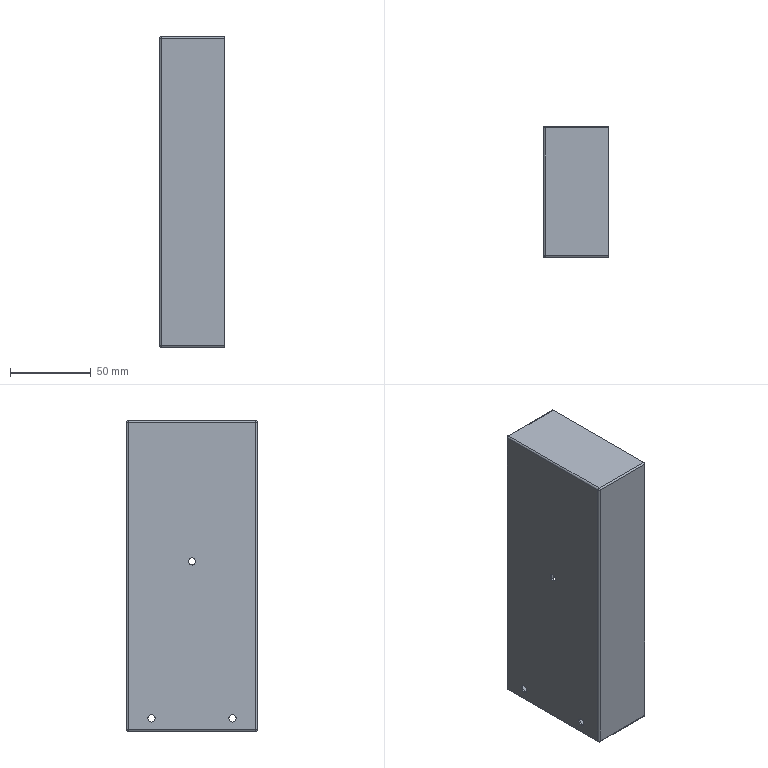Part | STEP file | FFH80-PL-018^FFH85-PL-M75-B3-01_three-axis module | 1 solid | 29 faces | box 40 x 81 x 192 mm | volume 36491 mm3 | cylinder 14 | plane 11 | sphere 4 | commonest cylinder face diameters 2 x8 4.5 x6
STEP:
#1=CARTESIAN_POINT('',(1.,0.,6.75));
#2=VERTEX_POINT('',#1);
#3=CARTESIAN_POINT('',(1.,0.,11.25));
#4=VERTEX_POINT('',#3);
#5=CARTESIAN_POINT('',(1.,0.,9.));
#6=DIRECTION('',(-1.,0.,0.));
#7=DIRECTION('',(0.,0.,1.));
#8=AXIS2_PLACEMENT_3D('',#5,#6,#7);
#9=CIRCLE('',#8,2.25);
#10=EDGE_CURVE('',#2,#4,#9,.T.);
#11=ORIENTED_EDGE('',*,*,#10,.F.);
#12=CARTESIAN_POINT('',(0.,0.,6.75));
#13=VERTEX_POINT('',#12);
#14=CARTESIAN_POINT('',(40.,0.,6.75));
#15=DIRECTION('',(-1.,0.,0.));
#16=VECTOR('',#15,1000.);
#17=LINE('',#14,#16);
#18=EDGE_CURVE('',#2,#13,#17,.T.);
#19=ORIENTED_EDGE('',*,*,#18,.T.);
#20=CARTESIAN_POINT('',(0.,0.,11.25));
#21=VERTEX_POINT('',#20);
#22=CARTESIAN_POINT('',(0.,0.,9.));
#23=DIRECTION('',(1.,0.,0.));
#24=DIRECTION('',(0.,0.,1.));
#25=AXIS2_PLACEMENT_3D('',#22,#23,#24);
#26=CIRCLE('',#25,2.25);
#27=EDGE_CURVE('',#21,#13,#26,.T.);
#28=ORIENTED_EDGE('',*,*,#27,.F.);
#29=CARTESIAN_POINT('',(40.,0.,11.25));
#30=DIRECTION('',(-1.,0.,0.));
#31=VECTOR('',#30,1000.);
#32=LINE('',#29,#31);
#33=EDGE_CURVE('',#4,#21,#32,.T.);
#34=ORIENTED_EDGE('',*,*,#33,.F.);
#35=EDGE_LOOP('',(#11,#19,#28,#34));
#36=FACE_OUTER_BOUND('',#35,.T.);
#37=CARTESIAN_POINT('',(40.,0.,9.));
#38=DIRECTION('',(-1.,0.,0.));
#39=DIRECTION('',(0.,0.,1.));
#40=AXIS2_PLACEMENT_3D('',#37,#38,#39);
#41=CYLINDRICAL_SURFACE('',#40,2.25);
#42=ADVANCED_FACE('',(#36),#41,.F.);
#43=CARTESIAN_POINT('',(1.,-25.,-90.25));
#44=VERTEX_POINT('',#43);
#45=CARTESIAN_POINT('',(1.,-25.,-85.75));
#46=VERTEX_POINT('',#45);
#47=CARTESIAN_POINT('',(1.,-25.,-88.));
#48=DIRECTION('',(-1.,0.,0.));
#49=DIRECTION('',(0.,0.,1.));
#50=AXIS2_PLACEMENT_3D('',#47,#48,#49);
#51=CIRCLE('',#50,2.25);
#52=EDGE_CURVE('',#44,#46,#51,.T.);
#53=ORIENTED_EDGE('',*,*,#52,.F.);
#54=CARTESIAN_POINT('',(0.,-25.,-90.25));
#55=VERTEX_POINT('',#54);
#56=CARTESIAN_POINT('',(40.,-25.,-90.25));
#57=DIRECTION('',(-1.,0.,0.));
#58=VECTOR('',#57,1000.);
#59=LINE('',#56,#58);
#60=EDGE_CURVE('',#44,#55,#59,.T.);
#61=ORIENTED_EDGE('',*,*,#60,.T.);
#62=CARTESIAN_POINT('',(0.,-25.,-85.75));
#63=VERTEX_POINT('',#62);
#64=CARTESIAN_POINT('',(0.,-25.,-88.));
#65=DIRECTION('',(1.,0.,0.));
#66=DIRECTION('',(0.,0.,1.));
#67=AXIS2_PLACEMENT_3D('',#64,#65,#66);
#68=CIRCLE('',#67,2.25);
#69=EDGE_CURVE('',#63,#55,#68,.T.);
#70=ORIENTED_EDGE('',*,*,#69,.F.);
#71=CARTESIAN_POINT('',(40.,-25.,-85.75));
#72=DIRECTION('',(-1.,0.,0.));
#73=VECTOR('',#72,1000.);
#74=LINE('',#71,#73);
#75=EDGE_CURVE('',#46,#63,#74,.T.);
#76=ORIENTED_EDGE('',*,*,#75,.F.);
#77=EDGE_LOOP('',(#53,#61,#70,#76));
#78=FACE_OUTER_BOUND('',#77,.T.);
#79=CARTESIAN_POINT('',(40.,-25.,-88.));
#80=DIRECTION('',(-1.,0.,0.));
#81=DIRECTION('',(0.,0.,1.));
#82=AXIS2_PLACEMENT_3D('',#79,#80,#81);
#83=CYLINDRICAL_SURFACE('',#82,2.25);
#84=ADVANCED_FACE('',(#78),#83,.F.);
#85=CARTESIAN_POINT('',(1.,25.,-90.25));
#86=VERTEX_POINT('',#85);
#87=CARTESIAN_POINT('',(1.,25.,-85.75));
#88=VERTEX_POINT('',#87);
#89=CARTESIAN_POINT('',(1.,25.,-88.));
#90=DIRECTION('',(-1.,0.,0.));
#91=DIRECTION('',(0.,0.,1.));
#92=AXIS2_PLACEMENT_3D('',#89,#90,#91);
#93=CIRCLE('',#92,2.25);
#94=EDGE_CURVE('',#86,#88,#93,.T.);
#95=ORIENTED_EDGE('',*,*,#94,.F.);
#96=CARTESIAN_POINT('',(0.,25.,-90.25));
#97=VERTEX_POINT('',#96);
#98=CARTESIAN_POINT('',(40.,25.,-90.25));
#99=DIRECTION('',(-1.,0.,0.));
#100=VECTOR('',#99,1000.);
#101=LINE('',#98,#100);
#102=EDGE_CURVE('',#86,#97,#101,.T.);
#103=ORIENTED_EDGE('',*,*,#102,.T.);
#104=CARTESIAN_POINT('',(0.,25.,-85.75));
#105=VERTEX_POINT('',#104);
#106=CARTESIAN_POINT('',(0.,25.,-88.));
#107=DIRECTION('',(1.,0.,0.));
#108=DIRECTION('',(0.,0.,1.));
#109=AXIS2_PLACEMENT_3D('',#106,#107,#108);
#110=CIRCLE('',#109,2.25);
#111=EDGE_CURVE('',#105,#97,#110,.T.);
#112=ORIENTED_EDGE('',*,*,#111,.F.);
#113=CARTESIAN_POINT('',(40.,25.,-85.75));
#114=DIRECTION('',(-1.,0.,0.));
#115=VECTOR('',#114,1000.);
#116=LINE('',#113,#115);
#117=EDGE_CURVE('',#88,#105,#116,.T.);
#118=ORIENTED_EDGE('',*,*,#117,.F.);
#119=EDGE_LOOP('',(#95,#103,#112,#118));
#120=FACE_OUTER_BOUND('',#119,.T.);
#121=CARTESIAN_POINT('',(40.,25.,-88.));
#122=DIRECTION('',(-1.,0.,0.));
#123=DIRECTION('',(0.,0.,1.));
#124=AXIS2_PLACEMENT_3D('',#121,#122,#123);
#125=CYLINDRICAL_SURFACE('',#124,2.25);
#126=ADVANCED_FACE('',(#120),#125,.F.);
#127=ORIENTED_EDGE('',*,*,#27,.T.);
#128=CARTESIAN_POINT('',(0.,0.,9.));
#129=DIRECTION('',(1.,0.,0.));
#130=DIRECTION('',(0.,0.,1.));
#131=AXIS2_PLACEMENT_3D('',#128,#129,#130);
#132=CIRCLE('',#131,2.25);
#133=EDGE_CURVE('',#13,#21,#132,.T.);
#134=ORIENTED_EDGE('',*,*,#133,.T.);
#135=EDGE_LOOP('',(#127,#134));
#136=FACE_BOUND('',#135,.T.);
#137=ORIENTED_EDGE('',*,*,#69,.T.);
#138=CARTESIAN_POINT('',(0.,-25.,-88.));
#139=DIRECTION('',(1.,0.,0.));
#140=DIRECTION('',(0.,0.,1.));
#141=AXIS2_PLACEMENT_3D('',#138,#139,#140);
#142=CIRCLE('',#141,2.25);
#143=EDGE_CURVE('',#55,#63,#142,.T.);
#144=ORIENTED_EDGE('',*,*,#143,.T.);
#145=EDGE_LOOP('',(#137,#144));
#146=FACE_BOUND('',#145,.T.);
#147=ORIENTED_EDGE('',*,*,#111,.T.);
#148=CARTESIAN_POINT('',(0.,25.,-88.));
#149=DIRECTION('',(1.,0.,0.));
#150=DIRECTION('',(0.,0.,1.));
#151=AXIS2_PLACEMENT_3D('',#148,#149,#150);
#152=CIRCLE('',#151,2.25);
#153=EDGE_CURVE('',#97,#105,#152,.T.);
#154=ORIENTED_EDGE('',*,*,#153,.T.);
#155=EDGE_LOOP('',(#147,#154));
#156=FACE_BOUND('',#155,.T.);
#157=CARTESIAN_POINT('',(0.,39.5,95.));
#158=VERTEX_POINT('',#157);
#159=CARTESIAN_POINT('',(0.,39.5,-95.));
#160=VERTEX_POINT('',#159);
#161=CARTESIAN_POINT('',(0.,39.5,0.));
#162=DIRECTION('',(0.,0.,-1.));
#163=VECTOR('',#162,1000.);
#164=LINE('',#161,#163);
#165=EDGE_CURVE('',#158,#160,#164,.T.);
#166=ORIENTED_EDGE('',*,*,#165,.T.);
#167=CARTESIAN_POINT('',(0.,-39.5,-95.));
#168=VERTEX_POINT('',#167);
#169=CARTESIAN_POINT('',(0.,0.,-95.));
#170=DIRECTION('',(0.,-1.,0.));
#171=VECTOR('',#170,1000.);
#172=LINE('',#169,#171);
#173=EDGE_CURVE('',#160,#168,#172,.T.);
#174=ORIENTED_EDGE('',*,*,#173,.T.);
#175=CARTESIAN_POINT('',(0.,-39.5,95.));
#176=VERTEX_POINT('',#175);
#177=CARTESIAN_POINT('',(0.,-39.5,0.));
#178=DIRECTION('',(0.,0.,1.));
#179=VECTOR('',#178,1000.);
#180=LINE('',#177,#179);
#181=EDGE_CURVE('',#168,#176,#180,.T.);
#182=ORIENTED_EDGE('',*,*,#181,.T.);
#183=CARTESIAN_POINT('',(0.,0.,95.));
#184=DIRECTION('',(0.,1.,0.));
#185=VECTOR('',#184,1000.);
#186=LINE('',#183,#185);
#187=EDGE_CURVE('',#176,#158,#186,.T.);
#188=ORIENTED_EDGE('',*,*,#187,.T.);
#189=EDGE_LOOP('',(#166,#174,#182,#188));
#190=FACE_OUTER_BOUND('',#189,.T.);
#191=CARTESIAN_POINT('',(0.,0.,0.));
#192=DIRECTION('',(-1.,0.,0.));
#193=DIRECTION('',(0.,0.,1.));
#194=AXIS2_PLACEMENT_3D('',#191,#192,#193);
#195=PLANE('',#194);
#196=ADVANCED_FACE('',(#136,#146,#156,#190),#195,.T.);
#197=ORIENTED_EDGE('',*,*,#18,.F.);
#198=CARTESIAN_POINT('',(1.,0.,9.));
#199=DIRECTION('',(-1.,0.,0.));
#200=DIRECTION('',(0.,0.,1.));
#201=AXIS2_PLACEMENT_3D('',#198,#199,#200);
#202=CIRCLE('',#201,2.25);
#203=EDGE_CURVE('',#4,#2,#202,.T.);
#204=ORIENTED_EDGE('',*,*,#203,.F.);
#205=ORIENTED_EDGE('',*,*,#33,.T.);
#206=ORIENTED_EDGE('',*,*,#133,.F.);
#207=EDGE_LOOP('',(#197,#204,#205,#206));
#208=FACE_OUTER_BOUND('',#207,.T.);
#209=CARTESIAN_POINT('',(40.,0.,9.));
#210=DIRECTION('',(-1.,0.,0.));
#211=DIRECTION('',(0.,0.,1.));
#212=AXIS2_PLACEMENT_3D('',#209,#210,#211);
#213=CYLINDRICAL_SURFACE('',#212,2.25);
#214=ADVANCED_FACE('',(#208),#213,.F.);
#215=ORIENTED_EDGE('',*,*,#60,.F.);
#216=CARTESIAN_POINT('',(1.,-25.,-88.));
#217=DIRECTION('',(-1.,0.,0.));
#218=DIRECTION('',(0.,0.,1.));
#219=AXIS2_PLACEMENT_3D('',#216,#217,#218);
#220=CIRCLE('',#219,2.25);
#221=EDGE_CURVE('',#46,#44,#220,.T.);
#222=ORIENTED_EDGE('',*,*,#221,.F.);
#223=ORIENTED_EDGE('',*,*,#75,.T.);
#224=ORIENTED_EDGE('',*,*,#143,.F.);
#225=EDGE_LOOP('',(#215,#222,#223,#224));
#226=FACE_OUTER_BOUND('',#225,.T.);
#227=CARTESIAN_POINT('',(40.,-25.,-88.));
#228=DIRECTION('',(-1.,0.,0.));
#229=DIRECTION('',(0.,0.,1.));
#230=AXIS2_PLACEMENT_3D('',#227,#228,#229);
#231=CYLINDRICAL_SURFACE('',#230,2.25);
#232=ADVANCED_FACE('',(#226),#231,.F.);
#233=ORIENTED_EDGE('',*,*,#102,.F.);
#234=CARTESIAN_POINT('',(1.,25.,-88.));
#235=DIRECTION('',(-1.,0.,0.));
#236=DIRECTION('',(0.,0.,1.));
#237=AXIS2_PLACEMENT_3D('',#234,#235,#236);
#238=CIRCLE('',#237,2.25);
#239=EDGE_CURVE('',#88,#86,#238,.T.);
#240=ORIENTED_EDGE('',*,*,#239,.F.);
#241=ORIENTED_EDGE('',*,*,#117,.T.);
#242=ORIENTED_EDGE('',*,*,#153,.F.);
#243=EDGE_LOOP('',(#233,#240,#241,#242));
#244=FACE_OUTER_BOUND('',#243,.T.);
#245=CARTESIAN_POINT('',(40.,25.,-88.));
#246=DIRECTION('',(-1.,0.,0.));
#247=DIRECTION('',(0.,0.,1.));
#248=AXIS2_PLACEMENT_3D('',#245,#246,#247);
#249=CYLINDRICAL_SURFACE('',#248,2.25);
#250=ADVANCED_FACE('',(#244),#249,.F.);
#251=CARTESIAN_POINT('',(1.,39.5,-96.));
#252=VERTEX_POINT('',#251);
#253=CARTESIAN_POINT('',(1.,39.5,-95.));
#254=DIRECTION('',(0.,-1.,0.));
#255=DIRECTION('',(0.,0.,-1.));
#256=AXIS2_PLACEMENT_3D('',#253,#254,#255);
#257=CIRCLE('',#256,1.);
#258=EDGE_CURVE('',#160,#252,#257,.T.);
#259=ORIENTED_EDGE('',*,*,#258,.T.);
#260=CARTESIAN_POINT('',(1.,-39.5,-96.));
#261=VERTEX_POINT('',#260);
#262=CARTESIAN_POINT('',(1.,40.5,-96.));
#263=DIRECTION('',(0.,-1.,0.));
#264=VECTOR('',#263,1000.);
#265=LINE('',#262,#264);
#266=EDGE_CURVE('',#252,#261,#265,.T.);
#267=ORIENTED_EDGE('',*,*,#266,.T.);
#268=CARTESIAN_POINT('',(1.,-39.5,-95.));
#269=DIRECTION('',(0.,1.,0.));
#270=DIRECTION('',(0.,0.,-1.));
#271=AXIS2_PLACEMENT_3D('',#268,#269,#270);
#272=CIRCLE('',#271,1.);
#273=EDGE_CURVE('',#261,#168,#272,.T.);
#274=ORIENTED_EDGE('',*,*,#273,.T.);
#275=ORIENTED_EDGE('',*,*,#173,.F.);
#276=EDGE_LOOP('',(#259,#267,#274,#275));
#277=FACE_OUTER_BOUND('',#276,.T.);
#278=CARTESIAN_POINT('',(1.,40.5,-95.));
#279=DIRECTION('',(0.,-1.,0.));
#280=DIRECTION('',(0.,0.,-1.));
#281=AXIS2_PLACEMENT_3D('',#278,#279,#280);
#282=CYLINDRICAL_SURFACE('',#281,1.);
#283=ADVANCED_FACE('',(#277),#282,.T.);
#284=CARTESIAN_POINT('',(1.,40.5,-95.));
#285=VERTEX_POINT('',#284);
#286=CARTESIAN_POINT('',(1.,39.5,-95.));
#287=DIRECTION('',(0.,0.,1.));
#288=DIRECTION('',(0.,1.,0.));
#289=AXIS2_PLACEMENT_3D('',#286,#287,#288);
#290=CIRCLE('',#289,1.);
#291=EDGE_CURVE('',#285,#160,#290,.T.);
#292=ORIENTED_EDGE('',*,*,#291,.T.);
#293=ORIENTED_EDGE('',*,*,#165,.F.);
#294=CARTESIAN_POINT('',(1.,40.5,95.));
#295=VERTEX_POINT('',#294);
#296=CARTESIAN_POINT('',(1.,39.5,95.));
#297=DIRECTION('',(0.,0.,-1.));
#298=DIRECTION('',(0.,1.,0.));
#299=AXIS2_PLACEMENT_3D('',#296,#297,#298);
#300=CIRCLE('',#299,1.);
#301=EDGE_CURVE('',#158,#295,#300,.T.);
#302=ORIENTED_EDGE('',*,*,#301,.T.);
#303=CARTESIAN_POINT('',(1.,40.5,-96.));
#304=DIRECTION('',(0.,0.,-1.));
#305=VECTOR('',#304,1000.);
#306=LINE('',#303,#305);
#307=EDGE_CURVE('',#295,#285,#306,.T.);
#308=ORIENTED_EDGE('',*,*,#307,.T.);
#309=EDGE_LOOP('',(#292,#293,#302,#308));
#310=FACE_OUTER_BOUND('',#309,.T.);
#311=CARTESIAN_POINT('',(1.,39.5,-96.));
#312=DIRECTION('',(0.,0.,-1.));
#313=DIRECTION('',(0.,1.,0.));
#314=AXIS2_PLACEMENT_3D('',#311,#312,#313);
#315=CYLINDRICAL_SURFACE('',#314,1.);
#316=ADVANCED_FACE('',(#310),#315,.T.);
#317=CARTESIAN_POINT('',(1.,39.5,96.));
#318=VERTEX_POINT('',#317);
#319=CARTESIAN_POINT('',(1.,39.5,95.));
#320=DIRECTION('',(0.,-1.,0.));
#321=DIRECTION('',(0.,0.,1.));
#322=AXIS2_PLACEMENT_3D('',#319,#320,#321);
#323=CIRCLE('',#322,1.);
#324=EDGE_CURVE('',#318,#158,#323,.T.);
#325=ORIENTED_EDGE('',*,*,#324,.T.);
#326=ORIENTED_EDGE('',*,*,#187,.F.);
#327=CARTESIAN_POINT('',(1.,-39.5,96.));
#328=VERTEX_POINT('',#327);
#329=CARTESIAN_POINT('',(1.,-39.5,95.));
#330=DIRECTION('',(0.,1.,0.));
#331=DIRECTION('',(0.,0.,1.));
#332=AXIS2_PLACEMENT_3D('',#329,#330,#331);
#333=CIRCLE('',#332,1.);
#334=EDGE_CURVE('',#176,#328,#333,.T.);
#335=ORIENTED_EDGE('',*,*,#334,.T.);
#336=CARTESIAN_POINT('',(1.,40.5,96.));
#337=DIRECTION('',(0.,1.,0.));
#338=VECTOR('',#337,1000.);
#339=LINE('',#336,#338);
#340=EDGE_CURVE('',#328,#318,#339,.T.);
#341=ORIENTED_EDGE('',*,*,#340,.T.);
#342=EDGE_LOOP('',(#325,#326,#335,#341));
#343=FACE_OUTER_BOUND('',#342,.T.);
#344=CARTESIAN_POINT('',(1.,40.5,95.));
#345=DIRECTION('',(0.,1.,0.));
#346=DIRECTION('',(0.,0.,1.));
#347=AXIS2_PLACEMENT_3D('',#344,#345,#346);
#348=CYLINDRICAL_SURFACE('',#347,1.);
#349=ADVANCED_FACE('',(#343),#348,.T.);
#350=CARTESIAN_POINT('',(1.,-40.5,-95.));
#351=VERTEX_POINT('',#350);
#352=CARTESIAN_POINT('',(1.,-39.5,-95.));
#353=DIRECTION('',(0.,0.,1.));
#354=DIRECTION('',(0.,-1.,0.));
#355=AXIS2_PLACEMENT_3D('',#352,#353,#354);
#356=CIRCLE('',#355,1.);
#357=EDGE_CURVE('',#168,#351,#356,.T.);
#358=ORIENTED_EDGE('',*,*,#357,.T.);
#359=CARTESIAN_POINT('',(1.,-40.5,95.));
#360=VERTEX_POINT('',#359);
#361=CARTESIAN_POINT('',(1.,-40.5,-96.));
#362=DIRECTION('',(0.,0.,1.));
#363=VECTOR('',#362,1000.);
#364=LINE('',#361,#363);
#365=EDGE_CURVE('',#351,#360,#364,.T.);
#366=ORIENTED_EDGE('',*,*,#365,.T.);
#367=CARTESIAN_POINT('',(1.,-39.5,95.));
#368=DIRECTION('',(0.,0.,-1.));
#369=DIRECTION('',(0.,-1.,0.));
#370=AXIS2_PLACEMENT_3D('',#367,#368,#369);
#371=CIRCLE('',#370,1.);
#372=EDGE_CURVE('',#360,#176,#371,.T.);
#373=ORIENTED_EDGE('',*,*,#372,.T.);
#374=ORIENTED_EDGE('',*,*,#181,.F.);
#375=EDGE_LOOP('',(#358,#366,#373,#374));
#376=FACE_OUTER_BOUND('',#375,.T.);
#377=CARTESIAN_POINT('',(1.,-39.5,-96.));
#378=DIRECTION('',(0.,0.,1.));
#379=DIRECTION('',(0.,-1.,0.));
#380=AXIS2_PLACEMENT_3D('',#377,#378,#379);
#381=CYLINDRICAL_SURFACE('',#380,1.);
#382=ADVANCED_FACE('',(#376),#381,.T.);
#383=ORIENTED_EDGE('',*,*,#203,.T.);
#384=ORIENTED_EDGE('',*,*,#10,.T.);
#385=EDGE_LOOP('',(#383,#384));
#386=FACE_BOUND('',#385,.T.);
#387=ORIENTED_EDGE('',*,*,#221,.T.);
#388=ORIENTED_EDGE('',*,*,#52,.T.);
#389=EDGE_LOOP('',(#387,#388));
#390=FACE_BOUND('',#389,.T.);
#391=ORIENTED_EDGE('',*,*,#239,.T.);
#392=ORIENTED_EDGE('',*,*,#94,.T.);
#393=EDGE_LOOP('',(#391,#392));
#394=FACE_BOUND('',#393,.T.);
#395=CARTESIAN_POINT('',(1.,39.5,-95.));
#396=VERTEX_POINT('',#395);
#397=CARTESIAN_POINT('',(1.,-39.5,-95.));
#398=VERTEX_POINT('',#397);
#399=CARTESIAN_POINT('',(1.,0.,-95.));
#400=DIRECTION('',(0.,-1.,0.));
#401=VECTOR('',#400,1000.);
#402=LINE('',#399,#401);
#403=EDGE_CURVE('',#396,#398,#402,.T.);
#404=ORIENTED_EDGE('',*,*,#403,.F.);
#405=CARTESIAN_POINT('',(1.,39.5,95.));
#406=VERTEX_POINT('',#405);
#407=CARTESIAN_POINT('',(1.,39.5,0.));
#408=DIRECTION('',(0.,0.,-1.));
#409=VECTOR('',#408,1000.);
#410=LINE('',#407,#409);
#411=EDGE_CURVE('',#406,#396,#410,.T.);
#412=ORIENTED_EDGE('',*,*,#411,.F.);
#413=CARTESIAN_POINT('',(1.,-39.5,95.));
#414=VERTEX_POINT('',#413);
#415=CARTESIAN_POINT('',(1.,0.,95.));
#416=DIRECTION('',(0.,1.,0.));
#417=VECTOR('',#416,1000.);
#418=LINE('',#415,#417);
#419=EDGE_CURVE('',#414,#406,#418,.T.);
#420=ORIENTED_EDGE('',*,*,#419,.F.);
#421=CARTESIAN_POINT('',(1.,-39.5,0.));
#422=DIRECTION('',(0.,0.,1.));
#423=VECTOR('',#422,1000.);
#424=LINE('',#421,#423);
#425=EDGE_CURVE('',#398,#414,#424,.T.);
#426=ORIENTED_EDGE('',*,*,#425,.F.);
#427=EDGE_LOOP('',(#404,#412,#420,#426));
#428=FACE_OUTER_BOUND('',#427,.T.);
#429=CARTESIAN_POINT('',(1.,0.,0.));
#430=DIRECTION('',(-1.,0.,0.));
#431=DIRECTION('',(0.,0.,1.));
#432=AXIS2_PLACEMENT_3D('',#429,#430,#431);
#433=PLANE('',#432);
#434=ADVANCED_FACE('',(#386,#390,#394,#428),#433,.F.);
#435=CARTESIAN_POINT('',(40.,39.5,-96.));
#436=VERTEX_POINT('',#435);
#437=CARTESIAN_POINT('',(40.,39.5,-96.));
#438=DIRECTION('',(-1.,0.,0.));
#439=VECTOR('',#438,1000.);
#440=LINE('',#437,#439);
#441=EDGE_CURVE('',#436,#252,#440,.T.);
#442=ORIENTED_EDGE('',*,*,#441,.F.);
#443=CARTESIAN_POINT('',(40.,-39.5,-96.));
#444=VERTEX_POINT('',#443);
#445=CARTESIAN_POINT('',(40.,40.5,-96.));
#446=DIRECTION('',(0.,1.,0.));
#447=VECTOR('',#446,1000.);
#448=LINE('',#445,#447);
#449=EDGE_CURVE('',#444,#436,#448,.T.);
#450=ORIENTED_EDGE('',*,*,#449,.F.);
#451=CARTESIAN_POINT('',(40.,-39.5,-96.));
#452=DIRECTION('',(1.,0.,0.));
#453=VECTOR('',#452,1000.);
#454=LINE('',#451,#453);
#455=EDGE_CURVE('',#261,#444,#454,.T.);
#456=ORIENTED_EDGE('',*,*,#455,.F.);
#457=ORIENTED_EDGE('',*,*,#266,.F.);
#458=EDGE_LOOP('',(#442,#450,#456,#457));
#459=FACE_OUTER_BOUND('',#458,.T.);
#460=CARTESIAN_POINT('',(40.,40.5,-96.));
#461=DIRECTION('',(0.,0.,1.));
#462=DIRECTION('',(0.,-1.,0.));
#463=AXIS2_PLACEMENT_3D('',#460,#461,#462);
#464=PLANE('',#463);
#465=ADVANCED_FACE('',(#459),#464,.F.);
#466=ORIENTED_EDGE('',*,*,#258,.F.);
#467=ORIENTED_EDGE('',*,*,#291,.F.);
#468=CARTESIAN_POINT('',(1.,39.5,-95.));
#469=DIRECTION('',(-1.,0.,0.));
#470=DIRECTION('',(0.,0.,-1.));
#471=AXIS2_PLACEMENT_3D('',#468,#469,#470);
#472=CIRCLE('',#471,1.);
#473=EDGE_CURVE('',#285,#252,#472,.T.);
#474=ORIENTED_EDGE('',*,*,#473,.T.);
#475=EDGE_LOOP('',(#466,#467,#474));
#476=FACE_OUTER_BOUND('',#475,.T.);
#477=CARTESIAN_POINT('',(1.,39.5,-95.));
#478=DIRECTION('',(0.,1.,0.));
#479=DIRECTION('',(0.,0.,-1.));
#480=AXIS2_PLACEMENT_3D('',#477,#478,#479);
#481=SPHERICAL_SURFACE('',#480,1.);
#482=ADVANCED_FACE('',(#476),#481,.T.);
#483=ORIENTED_EDGE('',*,*,#357,.F.);
#484=ORIENTED_EDGE('',*,*,#273,.F.);
#485=CARTESIAN_POINT('',(1.,-39.5,-95.));
#486=DIRECTION('',(-1.,0.,0.));
#487=DIRECTION('',(0.,-1.,0.));
#488=AXIS2_PLACEMENT_3D('',#485,#486,#487);
#489=CIRCLE('',#488,1.);
#490=EDGE_CURVE('',#261,#351,#489,.T.);
#491=ORIENTED_EDGE('',*,*,#490,.T.);
#492=EDGE_LOOP('',(#483,#484,#491));
#493=FACE_OUTER_BOUND('',#492,.T.);
#494=CARTESIAN_POINT('',(1.,-39.5,-95.));
#495=DIRECTION('',(0.,0.,-1.));
#496=DIRECTION('',(0.,-1.,0.));
#497=AXIS2_PLACEMENT_3D('',#494,#495,#496);
#498=SPHERICAL_SURFACE('',#497,1.);
#499=ADVANCED_FACE('',(#493),#498,.T.);
#500=CARTESIAN_POINT('',(40.,40.5,95.));
#501=VERTEX_POINT('',#500);
#502=CARTESIAN_POINT('',(40.,40.5,95.));
#503=DIRECTION('',(-1.,0.,0.));
#504=VECTOR('',#503,1000.);
#505=LINE('',#502,#504);
#506=EDGE_CURVE('',#501,#295,#505,.T.);
#507=ORIENTED_EDGE('',*,*,#506,.F.);
#508=CARTESIAN_POINT('',(40.,40.5,-95.));
#509=VERTEX_POINT('',#508);
#510=CARTESIAN_POINT('',(40.,40.5,-96.));
#511=DIRECTION('',(0.,0.,1.));
#512=VECTOR('',#511,1000.);
#513=LINE('',#510,#512);
#514=EDGE_CURVE('',#509,#501,#513,.T.);
#515=ORIENTED_EDGE('',*,*,#514,.F.);
#516=CARTESIAN_POINT('',(40.,40.5,-95.));
#517=DIRECTION('',(1.,0.,0.));
#518=VECTOR('',#517,1000.);
#519=LINE('',#516,#518);
#520=EDGE_CURVE('',#285,#509,#519,.T.);
#521=ORIENTED_EDGE('',*,*,#520,.F.);
#522=ORIENTED_EDGE('',*,*,#307,.F.);
#523=EDGE_LOOP('',(#507,#515,#521,#522));
#524=FACE_OUTER_BOUND('',#523,.T.);
#525=CARTESIAN_POINT('',(40.,40.5,-96.));
#526=DIRECTION('',(0.,-1.,0.));
#527=DIRECTION('',(0.,0.,-1.));
#528=AXIS2_PLACEMENT_3D('',#525,#526,#527);
#529=PLANE('',#528);
#530=ADVANCED_FACE('',(#524),#529,.F.);
#531=ORIENTED_EDGE('',*,*,#324,.F.);
#532=CARTESIAN_POINT('',(1.,39.5,95.));
#533=DIRECTION('',(-1.,0.,0.));
#534=DIRECTION('',(0.,1.,0.));
#535=AXIS2_PLACEMENT_3D('',#532,#533,#534);
#536=CIRCLE('',#535,1.);
#537=EDGE_CURVE('',#318,#295,#536,.T.);
#538=ORIENTED_EDGE('',*,*,#537,.T.);
#539=ORIENTED_EDGE('',*,*,#301,.F.);
#540=EDGE_LOOP('',(#531,#538,#539));
#541=FACE_OUTER_BOUND('',#540,.T.);
#542=CARTESIAN_POINT('',(1.,39.5,95.));
#543=DIRECTION('',(0.,0.,1.));
#544=DIRECTION('',(0.,1.,0.));
#545=AXIS2_PLACEMENT_3D('',#542,#543,#544);
#546=SPHERICAL_SURFACE('',#545,1.);
#547=ADVANCED_FACE('',(#541),#546,.T.);
#548=CARTESIAN_POINT('',(40.,-39.5,96.));
#549=VERTEX_POINT('',#548);
#550=CARTESIAN_POINT('',(40.,-39.5,96.));
#551=DIRECTION('',(-1.,0.,0.));
#552=VECTOR('',#551,1000.);
#553=LINE('',#550,#552);
#554=EDGE_CURVE('',#549,#328,#553,.T.);
#555=ORIENTED_EDGE('',*,*,#554,.F.);
#556=CARTESIAN_POINT('',(40.,39.5,96.));
#557=VERTEX_POINT('',#556);
#558=CARTESIAN_POINT('',(40.,40.5,96.));
#559=DIRECTION('',(0.,-1.,0.));
#560=VECTOR('',#559,1000.);
#561=LINE('',#558,#560);
#562=EDGE_CURVE('',#557,#549,#561,.T.);
#563=ORIENTED_EDGE('',*,*,#562,.F.);
#564=CARTESIAN_POINT('',(40.,39.5,96.));
#565=DIRECTION('',(1.,0.,0.));
#566=VECTOR('',#565,1000.);
#567=LINE('',#564,#566);
#568=EDGE_CURVE('',#318,#557,#567,.T.);
#569=ORIENTED_EDGE('',*,*,#568,.F.);
#570=ORIENTED_EDGE('',*,*,#340,.F.);
#571=EDGE_LOOP('',(#555,#563,#569,#570));
#572=FACE_OUTER_BOUND('',#571,.T.);
#573=CARTESIAN_POINT('',(40.,40.5,96.));
#574=DIRECTION('',(0.,0.,-1.));
#575=DIRECTION('',(0.,1.,0.));
#576=AXIS2_PLACEMENT_3D('',#573,#574,#575);
#577=PLANE('',#576);
#578=ADVANCED_FACE('',(#572),#577,.F.);
#579=ORIENTED_EDGE('',*,*,#334,.F.);
#580=ORIENTED_EDGE('',*,*,#372,.F.);
#581=CARTESIAN_POINT('',(1.,-39.5,95.));
#582=DIRECTION('',(-1.,0.,0.));
#583=DIRECTION('',(0.,0.,1.));
#584=AXIS2_PLACEMENT_3D('',#581,#582,#583);
#585=CIRCLE('',#584,1.);
#586=EDGE_CURVE('',#360,#328,#585,.T.);
#587=ORIENTED_EDGE('',*,*,#586,.T.);
#588=EDGE_LOOP('',(#579,#580,#587));
#589=FACE_OUTER_BOUND('',#588,.T.);
#590=CARTESIAN_POINT('',(1.,-39.5,95.));
#591=DIRECTION('',(0.,-1.,0.));
#592=DIRECTION('',(0.,0.,1.));
#593=AXIS2_PLACEMENT_3D('',#590,#591,#592);
#594=SPHERICAL_SURFACE('',#593,1.);
#595=ADVANCED_FACE('',(#589),#594,.T.);
#596=CARTESIAN_POINT('',(40.,-40.5,-95.));
#597=VERTEX_POINT('',#596);
#598=CARTESIAN_POINT('',(40.,-40.5,-95.));
#599=DIRECTION('',(-1.,0.,0.));
#600=VECTOR('',#599,1000.);
#601=LINE('',#598,#600);
#602=EDGE_CURVE('',#597,#351,#601,.T.);
#603=ORIENTED_EDGE('',*,*,#602,.F.);
#604=CARTESIAN_POINT('',(40.,-40.5,95.));
#605=VERTEX_POINT('',#604);
#606=CARTESIAN_POINT('',(40.,-40.5,-96.));
#607=DIRECTION('',(0.,0.,-1.));
#608=VECTOR('',#607,1000.);
#609=LINE('',#606,#608);
#610=EDGE_CURVE('',#605,#597,#609,.T.);
#611=ORIENTED_EDGE('',*,*,#610,.F.);
#612=CARTESIAN_POINT('',(40.,-40.5,95.));
#613=DIRECTION('',(1.,0.,0.));
#614=VECTOR('',#613,1000.);
#615=LINE('',#612,#614);
#616=EDGE_CURVE('',#360,#605,#615,.T.);
#617=ORIENTED_EDGE('',*,*,#616,.F.);
#618=ORIENTED_EDGE('',*,*,#365,.F.);
#619=EDGE_LOOP('',(#603,#611,#617,#618));
#620=FACE_OUTER_BOUND('',#619,.T.);
#621=CARTESIAN_POINT('',(40.,-40.5,-96.));
#622=DIRECTION('',(0.,1.,0.));
#623=DIRECTION('',(0.,0.,1.));
#624=AXIS2_PLACEMENT_3D('',#621,#622,#623);
#625=PLANE('',#624);
#626=ADVANCED_FACE('',(#620),#625,.F.);
#627=ORIENTED_EDGE('',*,*,#425,.T.);
#628=CARTESIAN_POINT('',(40.,-39.5,95.));
#629=VERTEX_POINT('',#628);
#630=CARTESIAN_POINT('',(40.,-39.5,95.));
#631=DIRECTION('',(1.,0.,0.));
#632=VECTOR('',#631,1000.);
#633=LINE('',#630,#632);
#634=EDGE_CURVE('',#414,#629,#633,.T.);
#635=ORIENTED_EDGE('',*,*,#634,.T.);
#636=CARTESIAN_POINT('',(40.,-39.5,-95.));
#637=VERTEX_POINT('',#636);
#638=CARTESIAN_POINT('',(40.,-39.5,-96.));
#639=DIRECTION('',(0.,0.,-1.));
#640=VECTOR('',#639,1000.);
#641=LINE('',#638,#640);
#642=EDGE_CURVE('',#629,#637,#641,.T.);
#643=ORIENTED_EDGE('',*,*,#642,.T.);
#644=CARTESIAN_POINT('',(40.,-39.5,-95.));
#645=DIRECTION('',(-1.,0.,0.));
#646=VECTOR('',#645,1000.);
#647=LINE('',#644,#646);
#648=EDGE_CURVE('',#637,#398,#647,.T.);
#649=ORIENTED_EDGE('',*,*,#648,.T.);
#650=EDGE_LOOP('',(#627,#635,#643,#649));
#651=FACE_OUTER_BOUND('',#650,.T.);
#652=CARTESIAN_POINT('',(40.,-39.5,-96.));
#653=DIRECTION('',(0.,1.,0.));
#654=DIRECTION('',(0.,0.,1.));
#655=AXIS2_PLACEMENT_3D('',#652,#653,#654);
#656=PLANE('',#655);
#657=ADVANCED_FACE('',(#651),#656,.T.);
#658=ORIENTED_EDGE('',*,*,#403,.T.);
#659=ORIENTED_EDGE('',*,*,#648,.F.);
#660=CARTESIAN_POINT('',(40.,39.5,-95.));
#661=VERTEX_POINT('',#660);
#662=CARTESIAN_POINT('',(40.,40.5,-95.));
#663=DIRECTION('',(0.,1.,0.));
#664=VECTOR('',#663,1000.);
#665=LINE('',#662,#664);
#666=EDGE_CURVE('',#637,#661,#665,.T.);
#667=ORIENTED_EDGE('',*,*,#666,.T.);
#668=CARTESIAN_POINT('',(40.,39.5,-95.));
#669=DIRECTION('',(-1.,0.,0.));
#670=VECTOR('',#669,1000.);
#671=LINE('',#668,#670);
#672=EDGE_CURVE('',#661,#396,#671,.T.);
#673=ORIENTED_EDGE('',*,*,#672,.T.);
#674=EDGE_LOOP('',(#658,#659,#667,#673));
#675=FACE_OUTER_BOUND('',#674,.T.);
#676=CARTESIAN_POINT('',(40.,40.5,-95.));
#677=DIRECTION('',(0.,0.,1.));
#678=DIRECTION('',(0.,-1.,0.));
#679=AXIS2_PLACEMENT_3D('',#676,#677,#678);
#680=PLANE('',#679);
#681=ADVANCED_FACE('',(#675),#680,.T.);
#682=ORIENTED_EDGE('',*,*,#411,.T.);
#683=ORIENTED_EDGE('',*,*,#672,.F.);
#684=CARTESIAN_POINT('',(40.,39.5,95.));
#685=VERTEX_POINT('',#684);
#686=CARTESIAN_POINT('',(40.,39.5,-96.));
#687=DIRECTION('',(0.,0.,1.));
#688=VECTOR('',#687,1000.);
#689=LINE('',#686,#688);
#690=EDGE_CURVE('',#661,#685,#689,.T.);
#691=ORIENTED_EDGE('',*,*,#690,.T.);
#692=CARTESIAN_POINT('',(40.,39.5,95.));
#693=DIRECTION('',(-1.,0.,0.));
#694=VECTOR('',#693,1000.);
#695=LINE('',#692,#694);
#696=EDGE_CURVE('',#685,#406,#695,.T.);
#697=ORIENTED_EDGE('',*,*,#696,.T.);
#698=EDGE_LOOP('',(#682,#683,#691,#697));
#699=FACE_OUTER_BOUND('',#698,.T.);
#700=CARTESIAN_POINT('',(40.,39.5,-96.));
#701=DIRECTION('',(0.,-1.,0.));
#702=DIRECTION('',(0.,0.,-1.));
#703=AXIS2_PLACEMENT_3D('',#700,#701,#702);
#704=PLANE('',#703);
#705=ADVANCED_FACE('',(#699),#704,.T.);
#706=ORIENTED_EDGE('',*,*,#419,.T.);
#707=ORIENTED_EDGE('',*,*,#696,.F.);
#708=CARTESIAN_POINT('',(40.,40.5,95.));
#709=DIRECTION('',(0.,-1.,0.));
#710=VECTOR('',#709,1000.);
#711=LINE('',#708,#710);
#712=EDGE_CURVE('',#685,#629,#711,.T.);
#713=ORIENTED_EDGE('',*,*,#712,.T.);
#714=ORIENTED_EDGE('',*,*,#634,.F.);
#715=EDGE_LOOP('',(#706,#707,#713,#714));
#716=FACE_OUTER_BOUND('',#715,.T.);
#717=CARTESIAN_POINT('',(40.,40.5,95.));
#718=DIRECTION('',(0.,0.,-1.));
#719=DIRECTION('',(0.,1.,0.));
#720=AXIS2_PLACEMENT_3D('',#717,#718,#719);
#721=PLANE('',#720);
#722=ADVANCED_FACE('',(#716),#721,.T.);
#723=ORIENTED_EDGE('',*,*,#441,.T.);
#724=ORIENTED_EDGE('',*,*,#473,.F.);
#725=ORIENTED_EDGE('',*,*,#520,.T.);
#726=CARTESIAN_POINT('',(40.,39.5,-95.));
#727=DIRECTION('',(-1.,0.,0.));
#728=DIRECTION('',(0.,0.,1.));
#729=AXIS2_PLACEMENT_3D('',#726,#727,#728);
#730=CIRCLE('',#729,1.);
#731=EDGE_CURVE('',#509,#436,#730,.T.);
#732=ORIENTED_EDGE('',*,*,#731,.T.);
#733=EDGE_LOOP('',(#723,#724,#725,#732));
#734=FACE_OUTER_BOUND('',#733,.T.);
#735=CARTESIAN_POINT('',(40.,39.5,-95.));
#736=DIRECTION('',(-1.,0.,0.));
#737=DIRECTION('',(0.,0.,1.));
#738=AXIS2_PLACEMENT_3D('',#735,#736,#737);
#739=CYLINDRICAL_SURFACE('',#738,1.);
#740=ADVANCED_FACE('',(#734),#739,.T.);
#741=ORIENTED_EDGE('',*,*,#562,.T.);
#742=CARTESIAN_POINT('',(40.,-39.5,95.));
#743=DIRECTION('',(-1.,0.,0.));
#744=DIRECTION('',(0.,0.,1.));
#745=AXIS2_PLACEMENT_3D('',#742,#743,#744);
#746=CIRCLE('',#745,1.);
#747=EDGE_CURVE('',#605,#549,#746,.T.);
#748=ORIENTED_EDGE('',*,*,#747,.F.);
#749=ORIENTED_EDGE('',*,*,#610,.T.);
#750=CARTESIAN_POINT('',(40.,-39.5,-95.));
#751=DIRECTION('',(-1.,0.,0.));
#752=DIRECTION('',(0.,0.,1.));
#753=AXIS2_PLACEMENT_3D('',#750,#751,#752);
#754=CIRCLE('',#753,1.);
#755=EDGE_CURVE('',#444,#597,#754,.T.);
#756=ORIENTED_EDGE('',*,*,#755,.F.);
#757=ORIENTED_EDGE('',*,*,#449,.T.);
#758=ORIENTED_EDGE('',*,*,#731,.F.);
#759=ORIENTED_EDGE('',*,*,#514,.T.);
#760=CARTESIAN_POINT('',(40.,39.5,95.));
#761=DIRECTION('',(-1.,0.,0.));
#762=DIRECTION('',(0.,0.,1.));
#763=AXIS2_PLACEMENT_3D('',#760,#761,#762);
#764=CIRCLE('',#763,1.);
#765=EDGE_CURVE('',#557,#501,#764,.T.);
#766=ORIENTED_EDGE('',*,*,#765,.F.);
#767=EDGE_LOOP('',(#741,#748,#749,#756,#757,#758,#759,#766));
#768=FACE_OUTER_BOUND('',#767,.T.);
#769=ORIENTED_EDGE('',*,*,#666,.F.);
#770=ORIENTED_EDGE('',*,*,#642,.F.);
#771=ORIENTED_EDGE('',*,*,#712,.F.);
#772=ORIENTED_EDGE('',*,*,#690,.F.);
#773=EDGE_LOOP('',(#769,#770,#771,#772));
#774=FACE_BOUND('',#773,.T.);
#775=CARTESIAN_POINT('',(40.,0.,0.));
#776=DIRECTION('',(-1.,0.,0.));
#777=DIRECTION('',(0.,0.,1.));
#778=AXIS2_PLACEMENT_3D('',#775,#776,#777);
#779=PLANE('',#778);
#780=ADVANCED_FACE('',(#768,#774),#779,.F.);
#781=ORIENTED_EDGE('',*,*,#602,.T.);
#782=ORIENTED_EDGE('',*,*,#490,.F.);
#783=ORIENTED_EDGE('',*,*,#455,.T.);
#784=ORIENTED_EDGE('',*,*,#755,.T.);
#785=EDGE_LOOP('',(#781,#782,#783,#784));
#786=FACE_OUTER_BOUND('',#785,.T.);
#787=CARTESIAN_POINT('',(40.,-39.5,-95.));
#788=DIRECTION('',(-1.,0.,0.));
#789=DIRECTION('',(0.,0.,1.));
#790=AXIS2_PLACEMENT_3D('',#787,#788,#789);
#791=CYLINDRICAL_SURFACE('',#790,1.);
#792=ADVANCED_FACE('',(#786),#791,.T.);
#793=ORIENTED_EDGE('',*,*,#506,.T.);
#794=ORIENTED_EDGE('',*,*,#537,.F.);
#795=ORIENTED_EDGE('',*,*,#568,.T.);
#796=ORIENTED_EDGE('',*,*,#765,.T.);
#797=EDGE_LOOP('',(#793,#794,#795,#796));
#798=FACE_OUTER_BOUND('',#797,.T.);
#799=CARTESIAN_POINT('',(40.,39.5,95.));
#800=DIRECTION('',(-1.,0.,0.));
#801=DIRECTION('',(0.,0.,1.));
#802=AXIS2_PLACEMENT_3D('',#799,#800,#801);
#803=CYLINDRICAL_SURFACE('',#802,1.);
#804=ADVANCED_FACE('',(#798),#803,.T.);
#805=ORIENTED_EDGE('',*,*,#554,.T.);
#806=ORIENTED_EDGE('',*,*,#586,.F.);
#807=ORIENTED_EDGE('',*,*,#616,.T.);
#808=ORIENTED_EDGE('',*,*,#747,.T.);
#809=EDGE_LOOP('',(#805,#806,#807,#808));
#810=FACE_OUTER_BOUND('',#809,.T.);
#811=CARTESIAN_POINT('',(40.,-39.5,95.));
#812=DIRECTION('',(-1.,0.,0.));
#813=DIRECTION('',(0.,0.,1.));
#814=AXIS2_PLACEMENT_3D('',#811,#812,#813);
#815=CYLINDRICAL_SURFACE('',#814,1.);
#816=ADVANCED_FACE('',(#810),#815,.T.);
#817=CLOSED_SHELL('',(#42,#84,#126,#196,#214,#232,#250,#283,#316,#349,#382,#434,#465,#482,#499,#530,#547,#578,#595,#626,#657,#681,#705,#722,#740,#780,#792,#804,#816));
#818=MANIFOLD_SOLID_BREP('',#817);
#819=CARTESIAN_POINT('',(0.,0.,0.));
#820=DIRECTION('',(0.,0.,1.));
#821=DIRECTION('',(1.,0.,0.));
#822=AXIS2_PLACEMENT_3D('',#819,#820,#821);
#823=(LENGTH_UNIT()NAMED_UNIT(*)SI_UNIT(.MILLI.,.METRE.));
#824=UNCERTAINTY_MEASURE_WITH_UNIT(LENGTH_MEASURE(0.00001),#823,'','');
#825=(NAMED_UNIT(*)PLANE_ANGLE_UNIT()SI_UNIT($,.RADIAN.));
#826=(NAMED_UNIT(*)SI_UNIT($,.STERADIAN.)SOLID_ANGLE_UNIT());
#827=(GEOMETRIC_REPRESENTATION_CONTEXT(3)GLOBAL_UNCERTAINTY_ASSIGNED_CONTEXT((#824))GLOBAL_UNIT_ASSIGNED_CONTEXT((#823,#825,#826))REPRESENTATION_CONTEXT('',''));
#828=ADVANCED_BREP_SHAPE_REPRESENTATION('',(#818,#822),#827);